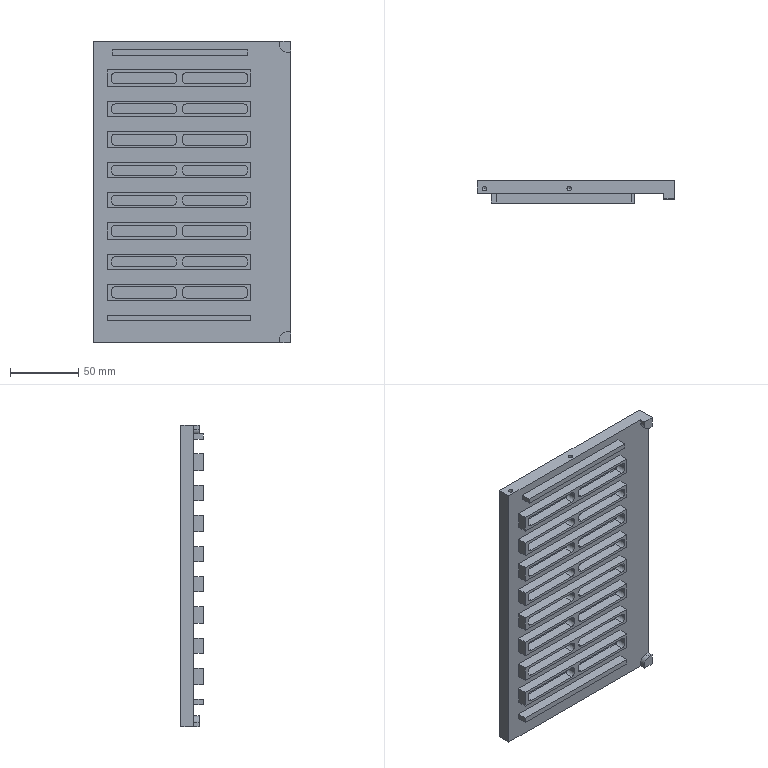NC program | NX | posted with a generic post | part box 144.5 x 16.5 x 221 mm
Lines 1769 to 2050 of 2050:
(THREAD_MILLING_2 , TOOL : THREAD_MILL)
N3524 T14 M6
N3526 G54
N3528 G17 G0 G90 X4.95 Y-6. S4500 M3
N3530 G43 Z20. H14
N3532 Z-9.175
N3534 G41 G94 G3 X4.83 Y-6.15 Z-9. I-0.06 J-0.075 F150. D14
N3536 X4.83 Y-6.15 Z-8.3 I0.12 J0.15
N3538 X4.95 Y-6. Z-8.125 I0.06 J0.075
N3540 G40
N3542 G0 Z-7.775
N3544 G41 G3 X4.83 Y-6.15 Z-7.6 I-0.06 J-0.075
N3546 X4.83 Y-6.15 Z-6.9 I0.12 J0.15
N3548 X4.95 Y-6. Z-6.725 I0.06 J0.075
N3550 G40
N3552 G0 Z-6.375
N3554 G41 G3 X4.83 Y-6.15 Z-6.2 I-0.06 J-0.075
N3556 X4.83 Y-6.15 Z-5.5 I0.12 J0.15
N3558 X4.95 Y-6. Z-5.325 I0.06 J0.075
N3560 G40
N3562 G0 Z-4.975
N3564 G41 G3 X4.83 Y-6.15 Z-4.8 I-0.06 J-0.075
N3566 X4.83 Y-6.15 Z-4.1 I0.12 J0.15
N3568 X4.95 Y-6. Z-3.925 I0.06 J0.075
N3570 G40
N3572 G0 Z-3.575
N3574 G41 G3 X4.83 Y-6.15 Z-3.4 I-0.06 J-0.075
N3576 X4.83 Y-6.15 Z-2.7 I0.12 J0.15
N3578 X4.95 Y-6. Z-2.525 I0.06 J0.075
N3580 G40
N3582 G0 Z-2.175
N3584 G41 G3 X4.83 Y-6.15 Z-2. I-0.06 J-0.075
N3586 X4.83 Y-6.15 Z-1.3 I0.12 J0.15
N3588 X4.95 Y-6. Z-1.125 I0.06 J0.075
N3590 G40
N3592 G0 Z-0.775
N3594 G41 G3 X4.83 Y-6.15 Z-0.6 I-0.06 J-0.075
N3596 X4.83 Y-6.15 Z0.1 I0.12 J0.15
N3598 X5.123 Y-6.083 Z0.3 R0.192
N3600 X4.95 Y-6. Z0.475 I-0.086 J0.042
N3602 G40
N3604 G0 Z-9.175
N3606 G41 G3 X4.758 Y-6.241 Z-9. I-0.096 J-0.121
N3608 X4.758 Y-6.241 Z-8.3 I0.192 J0.241
N3610 X4.95 Y-6. Z-8.125 I0.096 J0.121
N3612 G40
N3614 G0 Z-7.775
N3616 G41 G3 X4.758 Y-6.241 Z-7.6 I-0.096 J-0.121
N3618 X4.758 Y-6.241 Z-6.9 I0.192 J0.241
N3620 X4.95 Y-6. Z-6.725 I0.096 J0.121
N3622 G40
N3624 G0 Z-6.375
N3626 G41 G3 X4.758 Y-6.241 Z-6.2 I-0.096 J-0.121
N3628 X4.758 Y-6.241 Z-5.5 I0.192 J0.241
N3630 X4.95 Y-6. Z-5.325 I0.096 J0.121
N3632 G40
N3634 G0 Z-4.975
N3636 G41 G3 X4.758 Y-6.241 Z-4.8 I-0.096 J-0.121
N3638 X4.758 Y-6.241 Z-4.1 I0.192 J0.241
N3640 X4.95 Y-6. Z-3.925 I0.096 J0.121
N3642 G40
N3644 G0 Z-3.575
N3646 G41 G3 X4.758 Y-6.241 Z-3.4 I-0.096 J-0.121
N3648 X4.758 Y-6.241 Z-2.7 I0.192 J0.241
N3650 X4.95 Y-6. Z-2.525 I0.096 J0.121
N3652 G40
N3654 G0 Z-2.175
N3656 G41 G3 X4.758 Y-6.241 Z-2. I-0.096 J-0.121
N3658 X4.758 Y-6.241 Z-1.3 I0.192 J0.241
N3660 X4.95 Y-6. Z-1.125 I0.096 J0.121
N3662 G40
N3664 G0 Z-0.775
N3666 G41 G3 X4.758 Y-6.241 Z-0.6 I-0.096 J-0.121
N3668 X4.758 Y-6.241 Z0.1 I0.192 J0.241
N3670 X5.228 Y-6.134 Z0.3 R0.308
N3672 X4.95 Y-6. Z0.475 I-0.139 J0.067
N3674 G40
N3676 G0 Z-9.057
N3678 G41 G1 X4.686 Y-6.142
N3680 G3 X4.685 Y-6.332 Z-9. R0.122
N3682 X4.685 Y-6.332 Z-8.3 I0.265 J0.332
N3684 X4.871 Y-6.289 Z-8.243 R0.122
N3686 G40
N3688 G1 X4.95 Y-6.
N3690 G0 Z-7.657
N3692 G41 G1 X4.686 Y-6.142
N3694 G3 X4.685 Y-6.332 Z-7.6 R0.122
N3696 X4.685 Y-6.332 Z-6.9 I0.265 J0.332
N3698 X4.871 Y-6.289 Z-6.843 R0.122
N3700 G40
N3702 G1 X4.95 Y-6.
N3704 G0 Z-6.257
N3706 G41 G1 X4.686 Y-6.142
N3708 G3 X4.685 Y-6.332 Z-6.2 R0.122
N3710 X4.685 Y-6.332 Z-5.5 I0.265 J0.332
N3712 X4.871 Y-6.289 Z-5.443 R0.122
N3714 G40
N3716 G1 X4.95 Y-6.
N3718 G0 Z-4.857
N3720 G41 G1 X4.686 Y-6.142
N3722 G3 X4.685 Y-6.332 Z-4.8 R0.122
N3724 X4.685 Y-6.332 Z-4.1 I0.265 J0.332
N3726 X4.871 Y-6.289 Z-4.043 R0.122
N3728 G40
N3730 G1 X4.95 Y-6.
N3732 G0 Z-3.457
N3734 G41 G1 X4.686 Y-6.142
N3736 G3 X4.685 Y-6.332 Z-3.4 R0.122
N3738 X4.685 Y-6.332 Z-2.7 I0.265 J0.332
N3740 X4.871 Y-6.289 Z-2.643 R0.122
N3742 G40
N3744 G1 X4.95 Y-6.
N3746 G0 Z-2.057
N3748 G41 G1 X4.686 Y-6.142
N3750 G3 X4.685 Y-6.332 Z-2. R0.122
N3752 X4.685 Y-6.332 Z-1.3 I0.265 J0.332
N3754 X4.871 Y-6.289 Z-1.243 R0.122
N3756 G40
N3758 G1 X4.95 Y-6.
N3760 G0 Z-0.657
N3762 G41 G1 X4.686 Y-6.142
N3764 G3 X4.685 Y-6.332 Z-0.6 R0.122
N3766 X4.685 Y-6.332 Z0.1 I0.265 J0.332
N3768 X5.333 Y-6.184 Z0.3 R0.425
N3770 X5.25 Y-6.013 Z0.357 R0.122
N3772 G40
N3774 G1 X4.95 Y-6.
N3776 G0 Z20.
N3778 X66.95
N3780 Z-9.175
N3782 G41 G3 X66.83 Y-6.15 Z-9. I-0.06 J-0.075
N3784 X66.83 Y-6.15 Z-8.3 I0.12 J0.15
N3786 X66.95 Y-6. Z-8.125 I0.06 J0.075
N3788 G40
N3790 G0 Z-7.775
N3792 G41 G3 X66.83 Y-6.15 Z-7.6 I-0.06 J-0.075
N3794 X66.83 Y-6.15 Z-6.9 I0.12 J0.15
N3796 X66.95 Y-6. Z-6.725 I0.06 J0.075
N3798 G40
N3800 G0 Z-6.375
N3802 G41 G3 X66.83 Y-6.15 Z-6.2 I-0.06 J-0.075
N3804 X66.83 Y-6.15 Z-5.5 I0.12 J0.15
N3806 X66.95 Y-6. Z-5.325 I0.06 J0.075
N3808 G40
N3810 G0 Z-4.975
N3812 G41 G3 X66.83 Y-6.15 Z-4.8 I-0.06 J-0.075
N3814 X66.83 Y-6.15 Z-4.1 I0.12 J0.15
N3816 X66.95 Y-6. Z-3.925 I0.06 J0.075
N3818 G40
N3820 G0 Z-3.575
N3822 G41 G3 X66.83 Y-6.15 Z-3.4 I-0.06 J-0.075
N3824 X66.83 Y-6.15 Z-2.7 I0.12 J0.15
N3826 X66.95 Y-6. Z-2.525 I0.06 J0.075
N3828 G40
N3830 G0 Z-2.175
N3832 G41 G3 X66.83 Y-6.15 Z-2. I-0.06 J-0.075
N3834 X66.83 Y-6.15 Z-1.3 I0.12 J0.15
N3836 X66.95 Y-6. Z-1.125 I0.06 J0.075
N3838 G40
N3840 G0 Z-0.775
N3842 G41 G3 X66.83 Y-6.15 Z-0.6 I-0.06 J-0.075
N3844 X66.83 Y-6.15 Z0.1 I0.12 J0.15
N3846 X67.123 Y-6.083 Z0.3 R0.192
N3848 X66.95 Y-6. Z0.475 I-0.086 J0.042
N3850 G40
N3852 G0 Z-9.175
N3854 G41 G3 X66.758 Y-6.241 Z-9. I-0.096 J-0.121
N3856 X66.758 Y-6.241 Z-8.3 I0.192 J0.241
N3858 X66.95 Y-6. Z-8.125 I0.096 J0.121
N3860 G40
N3862 G0 Z-7.775
N3864 G41 G3 X66.758 Y-6.241 Z-7.6 I-0.096 J-0.121
N3866 X66.758 Y-6.241 Z-6.9 I0.192 J0.241
N3868 X66.95 Y-6. Z-6.725 I0.096 J0.121
N3870 G40
N3872 G0 Z-6.375
N3874 G41 G3 X66.758 Y-6.241 Z-6.2 I-0.096 J-0.121
N3876 X66.758 Y-6.241 Z-5.5 I0.192 J0.241
N3878 X66.95 Y-6. Z-5.325 I0.096 J0.121
N3880 G40
N3882 G0 Z-4.975
N3884 G41 G3 X66.758 Y-6.241 Z-4.8 I-0.096 J-0.121
N3886 X66.758 Y-6.241 Z-4.1 I0.192 J0.241
N3888 X66.95 Y-6. Z-3.925 I0.096 J0.121
N3890 G40
N3892 G0 Z-3.575
N3894 G41 G3 X66.758 Y-6.241 Z-3.4 I-0.096 J-0.121
N3896 X66.758 Y-6.241 Z-2.7 I0.192 J0.241
N3898 X66.95 Y-6. Z-2.525 I0.096 J0.121
N3900 G40
N3902 G0 Z-2.175
N3904 G41 G3 X66.758 Y-6.241 Z-2. I-0.096 J-0.121
N3906 X66.758 Y-6.241 Z-1.3 I0.192 J0.241
N3908 X66.95 Y-6. Z-1.125 I0.096 J0.121
N3910 G40
N3912 G0 Z-0.775
N3914 G41 G3 X66.758 Y-6.241 Z-0.6 I-0.096 J-0.121
N3916 X66.758 Y-6.241 Z0.1 I0.192 J0.241
N3918 X67.228 Y-6.134 Z0.3 R0.308
N3920 X66.95 Y-6. Z0.475 I-0.139 J0.067
N3922 G40
N3924 G0 Z-9.057
N3926 G41 G1 X66.686 Y-6.142
N3928 G3 X66.685 Y-6.332 Z-9. R0.122
N3930 X66.685 Y-6.332 Z-8.3 I0.265 J0.332
N3932 X66.871 Y-6.289 Z-8.243 R0.122
N3934 G40
N3936 G1 X66.95 Y-6.
N3938 G0 Z-7.657
N3940 G41 G1 X66.686 Y-6.142
N3942 G3 X66.685 Y-6.332 Z-7.6 R0.122
N3944 X66.685 Y-6.332 Z-6.9 I0.265 J0.332
N3946 X66.871 Y-6.289 Z-6.843 R0.122
N3948 G40
N3950 G1 X66.95 Y-6.
N3952 G0 Z-6.257
N3954 G41 G1 X66.686 Y-6.142
N3956 G3 X66.685 Y-6.332 Z-6.2 R0.122
N3958 X66.685 Y-6.332 Z-5.5 I0.265 J0.332
N3960 X66.871 Y-6.289 Z-5.443 R0.122
N3962 G40
N3964 G1 X66.95 Y-6.
N3966 G0 Z-4.857
N3968 G41 G1 X66.686 Y-6.142
N3970 G3 X66.685 Y-6.332 Z-4.8 R0.122
N3972 X66.685 Y-6.332 Z-4.1 I0.265 J0.332
N3974 X66.871 Y-6.289 Z-4.043 R0.122
N3976 G40
N3978 G1 X66.95 Y-6.
N3980 G0 Z-3.457
N3982 G41 G1 X66.686 Y-6.142
N3984 G3 X66.685 Y-6.332 Z-3.4 R0.122
N3986 X66.685 Y-6.332 Z-2.7 I0.265 J0.332
N3988 X66.871 Y-6.289 Z-2.643 R0.122
N3990 G40
N3992 G1 X66.95 Y-6.
N3994 G0 Z-2.057
N3996 G41 G1 X66.686 Y-6.142
N3998 G3 X66.685 Y-6.332 Z-2. R0.122
N4000 X66.685 Y-6.332 Z-1.3 I0.265 J0.332
N4002 X66.871 Y-6.289 Z-1.243 R0.122
N4004 G40
N4006 G1 X66.95 Y-6.
N4008 G0 Z-0.657
N4010 G41 G1 X66.686 Y-6.142
N4012 G3 X66.685 Y-6.332 Z-0.6 R0.122
N4014 X66.685 Y-6.332 Z0.1 I0.265 J0.332
N4016 X67.333 Y-6.184 Z0.3 R0.425
N4018 X67.25 Y-6.013 Z0.357 R0.122
N4020 G40
N4022 G1 X66.95 Y-6.
N4024 G0 Z20.
N4026 M5
(PLANAR_MILL_10_COPY_1 , TOOL : D16-48-D16-100-3T-FINISH)
N4028 T15 M6
N4030 G54
N4032 G17 G0 G90 X88.25 Y-7. S3500 M3
N4034 G43 Z20. H15
N4036 Z3.03
N4038 G94 G1 Z0.03 F800.
N4040 X72.25
N4042 X-72.25
N4044 X-88.25
N4046 Z3.03
N4048 G0 Z20.
(PLANAR_MILL_10_COPY_1_COPY , TOOL : D16-48-D16-100-3T-FINISH)
N4050 X88.25
N4052 Z3.
N4054 G1 Z0.
N4056 X72.25
N4058 X-72.25
N4060 X-88.25
N4062 Z3.
N4064 G0 Z20.
N4066 M5
N4068 M2